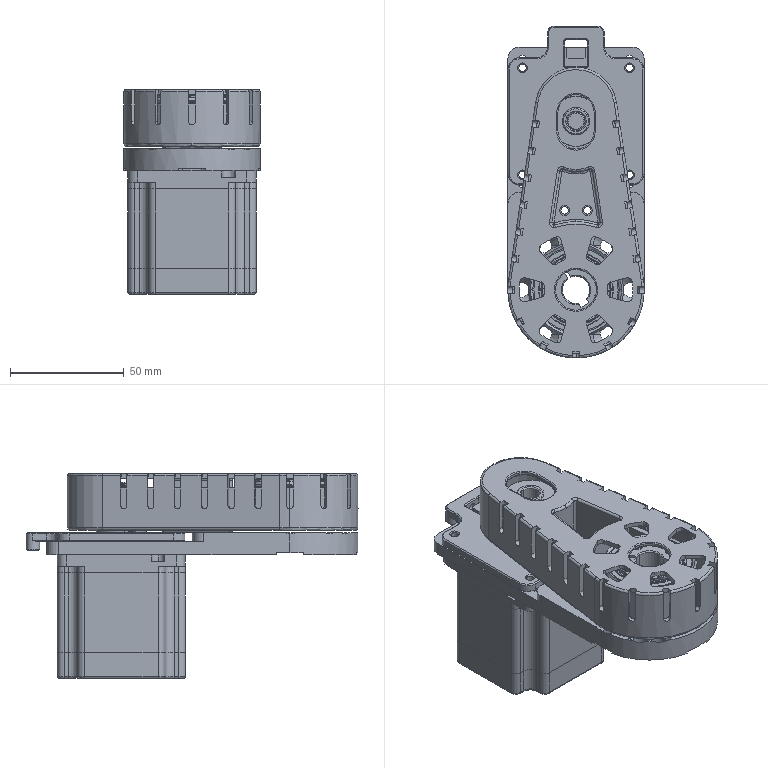Part | STEP file | Copy of CZ031-57 side link 2:1(60-60N)^K50A-1H20-S(formula driven)-L300-motor left- | 15 solids | 1305 faces | box 60 x 146.25 x 90.3 mm | volume 270957 mm3 | cylinder 689 | plane 345 | cone 167 | spline 91 | torus 13 | commonest cylinder face diameters 0.6 x162 1.82 x90 2 x64 37.44 x40 4 x32 6 x32